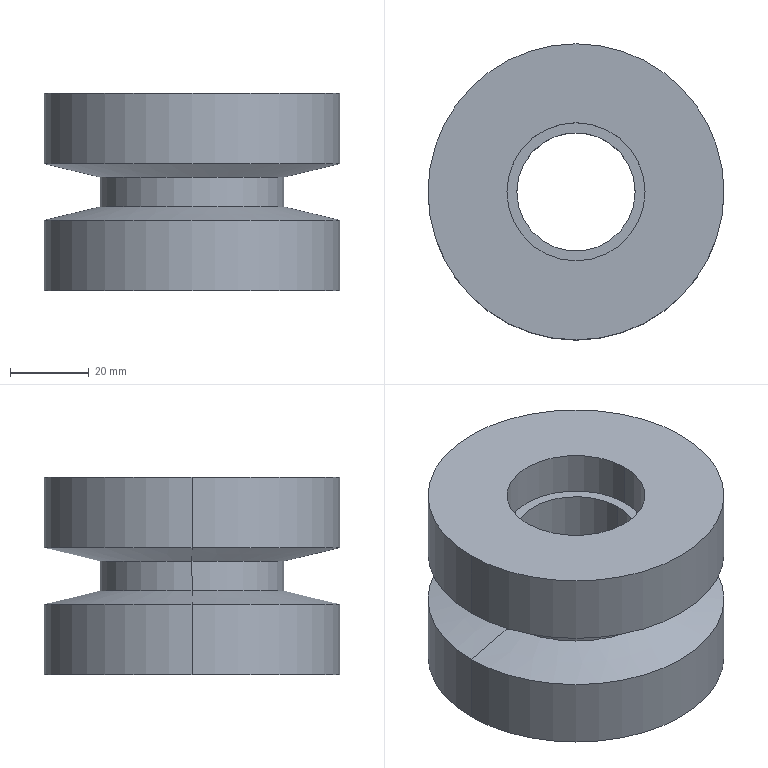Part | SolidWorks | features ICE 2, Extrusion 1, RevCut 1 | 1 solid | 20 faces | box 75 x 75 x 50 mm | volume 149506 mm3 | cylinder 12 | cone 4 | plane 4 | commonest cylinder face diameters 35 x4 75 x4 30 x2 46.5 x2
STEP:
#1=CARTESIAN_POINT('',(17.5,0.,11.));
#2=VERTEX_POINT('',#1);
#3=CARTESIAN_POINT('',(-17.5,0.,11.));
#4=VERTEX_POINT('',#3);
#5=CARTESIAN_POINT('',(0.,0.,11.));
#6=DIRECTION('',(0.,0.,-1.));
#7=DIRECTION('',(-1.,0.,0.));
#8=AXIS2_PLACEMENT_3D('',#5,#6,#7);
#9=CIRCLE('',#8,17.5);
#10=EDGE_CURVE('',#2,#4,#9,.T.);
#11=ORIENTED_EDGE('',*,*,#10,.F.);
#12=CARTESIAN_POINT('',(17.5,0.,0.));
#13=VERTEX_POINT('',#12);
#14=CARTESIAN_POINT('',(17.5,0.,11.));
#15=DIRECTION('',(0.,0.,-1.));
#16=VECTOR('',#15,1000.);
#17=LINE('',#14,#16);
#18=EDGE_CURVE('',#2,#13,#17,.T.);
#19=ORIENTED_EDGE('',*,*,#18,.T.);
#20=CARTESIAN_POINT('',(-17.5,0.,0.));
#21=VERTEX_POINT('',#20);
#22=CARTESIAN_POINT('',(0.,0.,0.));
#23=DIRECTION('',(0.,0.,-1.));
#24=DIRECTION('',(-1.,0.,0.));
#25=AXIS2_PLACEMENT_3D('',#22,#23,#24);
#26=CIRCLE('',#25,17.5);
#27=EDGE_CURVE('',#13,#21,#26,.T.);
#28=ORIENTED_EDGE('',*,*,#27,.T.);
#29=CARTESIAN_POINT('',(-17.5,0.,11.));
#30=DIRECTION('',(0.,0.,-1.));
#31=VECTOR('',#30,1000.);
#32=LINE('',#29,#31);
#33=EDGE_CURVE('',#4,#21,#32,.T.);
#34=ORIENTED_EDGE('',*,*,#33,.F.);
#35=EDGE_LOOP('',(#11,#19,#28,#34));
#36=FACE_OUTER_BOUND('',#35,.T.);
#37=CARTESIAN_POINT('',(0.,0.,11.));
#38=DIRECTION('',(0.,0.,-1.));
#39=DIRECTION('',(-1.,0.,0.));
#40=AXIS2_PLACEMENT_3D('',#37,#38,#39);
#41=CYLINDRICAL_SURFACE('',#40,17.5);
#42=ADVANCED_FACE('',(#36),#41,.F.);
#43=CARTESIAN_POINT('',(-17.5,0.,39.));
#44=VERTEX_POINT('',#43);
#45=CARTESIAN_POINT('',(17.5,0.,39.));
#46=VERTEX_POINT('',#45);
#47=CARTESIAN_POINT('',(0.,0.,39.));
#48=DIRECTION('',(0.,0.,1.));
#49=DIRECTION('',(1.,0.,0.));
#50=AXIS2_PLACEMENT_3D('',#47,#48,#49);
#51=CIRCLE('',#50,17.5);
#52=EDGE_CURVE('',#44,#46,#51,.T.);
#53=ORIENTED_EDGE('',*,*,#52,.F.);
#54=CARTESIAN_POINT('',(-17.5,0.,50.));
#55=VERTEX_POINT('',#54);
#56=CARTESIAN_POINT('',(-17.5,0.,39.));
#57=DIRECTION('',(0.,0.,1.));
#58=VECTOR('',#57,1000.);
#59=LINE('',#56,#58);
#60=EDGE_CURVE('',#44,#55,#59,.T.);
#61=ORIENTED_EDGE('',*,*,#60,.T.);
#62=CARTESIAN_POINT('',(17.5,0.,50.));
#63=VERTEX_POINT('',#62);
#64=CARTESIAN_POINT('',(0.,0.,50.));
#65=DIRECTION('',(0.,0.,1.));
#66=DIRECTION('',(1.,0.,0.));
#67=AXIS2_PLACEMENT_3D('',#64,#65,#66);
#68=CIRCLE('',#67,17.5);
#69=EDGE_CURVE('',#55,#63,#68,.T.);
#70=ORIENTED_EDGE('',*,*,#69,.T.);
#71=CARTESIAN_POINT('',(17.5,0.,39.));
#72=DIRECTION('',(0.,0.,1.));
#73=VECTOR('',#72,1000.);
#74=LINE('',#71,#73);
#75=EDGE_CURVE('',#46,#63,#74,.T.);
#76=ORIENTED_EDGE('',*,*,#75,.F.);
#77=EDGE_LOOP('',(#53,#61,#70,#76));
#78=FACE_OUTER_BOUND('',#77,.T.);
#79=CARTESIAN_POINT('',(0.,0.,39.));
#80=DIRECTION('',(0.,0.,1.));
#81=DIRECTION('',(1.,0.,0.));
#82=AXIS2_PLACEMENT_3D('',#79,#80,#81);
#83=CYLINDRICAL_SURFACE('',#82,17.5);
#84=ADVANCED_FACE('',(#78),#83,.F.);
#85=CARTESIAN_POINT('',(-23.25,0.,28.75));
#86=VERTEX_POINT('',#85);
#87=CARTESIAN_POINT('',(23.25,0.,28.75));
#88=VERTEX_POINT('',#87);
#89=CARTESIAN_POINT('',(0.,0.,28.75));
#90=DIRECTION('',(0.,0.,-1.));
#91=DIRECTION('',(-1.,0.,0.));
#92=AXIS2_PLACEMENT_3D('',#89,#90,#91);
#93=CIRCLE('',#92,23.25);
#94=EDGE_CURVE('',#86,#88,#93,.T.);
#95=ORIENTED_EDGE('',*,*,#94,.T.);
#96=CARTESIAN_POINT('',(23.25,0.,21.25));
#97=VERTEX_POINT('',#96);
#98=CARTESIAN_POINT('',(23.25,0.,0.));
#99=DIRECTION('',(0.,0.,-1.));
#100=VECTOR('',#99,1000.);
#101=LINE('',#98,#100);
#102=EDGE_CURVE('',#88,#97,#101,.T.);
#103=ORIENTED_EDGE('',*,*,#102,.T.);
#104=CARTESIAN_POINT('',(-23.25,0.,21.25));
#105=VERTEX_POINT('',#104);
#106=CARTESIAN_POINT('',(0.,0.,21.25));
#107=DIRECTION('',(0.,0.,-1.));
#108=DIRECTION('',(-1.,0.,0.));
#109=AXIS2_PLACEMENT_3D('',#106,#107,#108);
#110=CIRCLE('',#109,23.25);
#111=EDGE_CURVE('',#105,#97,#110,.T.);
#112=ORIENTED_EDGE('',*,*,#111,.F.);
#113=CARTESIAN_POINT('',(-23.25,0.,0.));
#114=DIRECTION('',(0.,0.,-1.));
#115=VECTOR('',#114,1000.);
#116=LINE('',#113,#115);
#117=EDGE_CURVE('',#86,#105,#116,.T.);
#118=ORIENTED_EDGE('',*,*,#117,.F.);
#119=EDGE_LOOP('',(#95,#103,#112,#118));
#120=FACE_OUTER_BOUND('',#119,.T.);
#121=CARTESIAN_POINT('',(0.,0.,0.));
#122=DIRECTION('',(0.,0.,-1.));
#123=DIRECTION('',(-1.,0.,0.));
#124=AXIS2_PLACEMENT_3D('',#121,#122,#123);
#125=CYLINDRICAL_SURFACE('',#124,23.25);
#126=ADVANCED_FACE('',(#120),#125,.T.);
#127=ORIENTED_EDGE('',*,*,#94,.F.);
#128=CARTESIAN_POINT('',(-37.5,0.,32.171));
#129=VERTEX_POINT('',#128);
#130=CARTESIAN_POINT('',(-38.25,0.,32.351));
#131=DIRECTION('',(-0.9724,0.,0.2334));
#132=VECTOR('',#131,1000.);
#133=LINE('',#130,#132);
#134=EDGE_CURVE('',#86,#129,#133,.T.);
#135=ORIENTED_EDGE('',*,*,#134,.T.);
#136=CARTESIAN_POINT('',(37.5,0.,32.171));
#137=VERTEX_POINT('',#136);
#138=CARTESIAN_POINT('',(0.,0.,32.171));
#139=DIRECTION('',(0.,0.,1.));
#140=DIRECTION('',(1.,0.,0.));
#141=AXIS2_PLACEMENT_3D('',#138,#139,#140);
#142=CIRCLE('',#141,37.5);
#143=EDGE_CURVE('',#137,#129,#142,.T.);
#144=ORIENTED_EDGE('',*,*,#143,.F.);
#145=CARTESIAN_POINT('',(38.25,0.,32.351));
#146=DIRECTION('',(0.9724,0.,0.2334));
#147=VECTOR('',#146,1000.);
#148=LINE('',#145,#147);
#149=EDGE_CURVE('',#88,#137,#148,.T.);
#150=ORIENTED_EDGE('',*,*,#149,.F.);
#151=EDGE_LOOP('',(#127,#135,#144,#150));
#152=FACE_OUTER_BOUND('',#151,.T.);
#153=CARTESIAN_POINT('',(0.,0.,32.351));
#154=DIRECTION('',(0.,0.,1.));
#155=DIRECTION('',(1.,0.,0.));
#156=AXIS2_PLACEMENT_3D('',#153,#154,#155);
#157=CONICAL_SURFACE('',#156,38.25,1.335);
#158=ADVANCED_FACE('',(#152),#157,.T.);
#159=ORIENTED_EDGE('',*,*,#111,.T.);
#160=CARTESIAN_POINT('',(37.5,0.,17.829));
#161=VERTEX_POINT('',#160);
#162=CARTESIAN_POINT('',(23.25,0.,21.25));
#163=DIRECTION('',(0.9724,0.,-0.2334));
#164=VECTOR('',#163,1000.);
#165=LINE('',#162,#164);
#166=EDGE_CURVE('',#97,#161,#165,.T.);
#167=ORIENTED_EDGE('',*,*,#166,.T.);
#168=CARTESIAN_POINT('',(-37.5,0.,17.829));
#169=VERTEX_POINT('',#168);
#170=CARTESIAN_POINT('',(0.,0.,17.829));
#171=DIRECTION('',(0.,0.,-1.));
#172=DIRECTION('',(-1.,0.,0.));
#173=AXIS2_PLACEMENT_3D('',#170,#171,#172);
#174=CIRCLE('',#173,37.5);
#175=EDGE_CURVE('',#169,#161,#174,.T.);
#176=ORIENTED_EDGE('',*,*,#175,.F.);
#177=CARTESIAN_POINT('',(-23.25,0.,21.25));
#178=DIRECTION('',(-0.9724,0.,-0.2334));
#179=VECTOR('',#178,1000.);
#180=LINE('',#177,#179);
#181=EDGE_CURVE('',#105,#169,#180,.T.);
#182=ORIENTED_EDGE('',*,*,#181,.F.);
#183=EDGE_LOOP('',(#159,#167,#176,#182));
#184=FACE_OUTER_BOUND('',#183,.T.);
#185=CARTESIAN_POINT('',(0.,0.,21.25));
#186=DIRECTION('',(0.,0.,-1.));
#187=DIRECTION('',(-1.,0.,0.));
#188=AXIS2_PLACEMENT_3D('',#185,#186,#187);
#189=CONICAL_SURFACE('',#188,23.25,1.335);
#190=ADVANCED_FACE('',(#184),#189,.T.);
#191=CARTESIAN_POINT('',(37.5,0.,50.));
#192=VERTEX_POINT('',#191);
#193=CARTESIAN_POINT('',(-37.5,0.,50.));
#194=VERTEX_POINT('',#193);
#195=CARTESIAN_POINT('',(0.,0.,50.));
#196=DIRECTION('',(0.,0.,1.));
#197=DIRECTION('',(1.,0.,0.));
#198=AXIS2_PLACEMENT_3D('',#195,#196,#197);
#199=CIRCLE('',#198,37.5);
#200=EDGE_CURVE('',#192,#194,#199,.T.);
#201=ORIENTED_EDGE('',*,*,#200,.F.);
#202=CARTESIAN_POINT('',(37.5,0.,50.));
#203=DIRECTION('',(0.,0.,-1.));
#204=VECTOR('',#203,1000.);
#205=LINE('',#202,#204);
#206=EDGE_CURVE('',#192,#137,#205,.T.);
#207=ORIENTED_EDGE('',*,*,#206,.T.);
#208=ORIENTED_EDGE('',*,*,#143,.T.);
#209=CARTESIAN_POINT('',(-37.5,0.,50.));
#210=DIRECTION('',(0.,0.,-1.));
#211=VECTOR('',#210,1000.);
#212=LINE('',#209,#211);
#213=EDGE_CURVE('',#194,#129,#212,.T.);
#214=ORIENTED_EDGE('',*,*,#213,.F.);
#215=EDGE_LOOP('',(#201,#207,#208,#214));
#216=FACE_OUTER_BOUND('',#215,.T.);
#217=CARTESIAN_POINT('',(0.,0.,50.));
#218=DIRECTION('',(0.,0.,-1.));
#219=DIRECTION('',(-1.,0.,0.));
#220=AXIS2_PLACEMENT_3D('',#217,#218,#219);
#221=CYLINDRICAL_SURFACE('',#220,37.5);
#222=ADVANCED_FACE('',(#216),#221,.T.);
#223=ORIENTED_EDGE('',*,*,#175,.T.);
#224=CARTESIAN_POINT('',(37.5,0.,0.));
#225=VERTEX_POINT('',#224);
#226=CARTESIAN_POINT('',(37.5,0.,50.));
#227=DIRECTION('',(0.,0.,-1.));
#228=VECTOR('',#227,1000.);
#229=LINE('',#226,#228);
#230=EDGE_CURVE('',#161,#225,#229,.T.);
#231=ORIENTED_EDGE('',*,*,#230,.T.);
#232=CARTESIAN_POINT('',(-37.5,0.,0.));
#233=VERTEX_POINT('',#232);
#234=CARTESIAN_POINT('',(0.,0.,0.));
#235=DIRECTION('',(0.,0.,1.));
#236=DIRECTION('',(1.,0.,0.));
#237=AXIS2_PLACEMENT_3D('',#234,#235,#236);
#238=CIRCLE('',#237,37.5);
#239=EDGE_CURVE('',#225,#233,#238,.T.);
#240=ORIENTED_EDGE('',*,*,#239,.T.);
#241=CARTESIAN_POINT('',(-37.5,0.,50.));
#242=DIRECTION('',(0.,0.,-1.));
#243=VECTOR('',#242,1000.);
#244=LINE('',#241,#243);
#245=EDGE_CURVE('',#169,#233,#244,.T.);
#246=ORIENTED_EDGE('',*,*,#245,.F.);
#247=EDGE_LOOP('',(#223,#231,#240,#246));
#248=FACE_OUTER_BOUND('',#247,.T.);
#249=CARTESIAN_POINT('',(0.,0.,50.));
#250=DIRECTION('',(0.,0.,-1.));
#251=DIRECTION('',(-1.,0.,0.));
#252=AXIS2_PLACEMENT_3D('',#249,#250,#251);
#253=CYLINDRICAL_SURFACE('',#252,37.5);
#254=ADVANCED_FACE('',(#248),#253,.T.);
#255=CARTESIAN_POINT('',(-15.,0.,39.));
#256=VERTEX_POINT('',#255);
#257=CARTESIAN_POINT('',(15.,0.,39.));
#258=VERTEX_POINT('',#257);
#259=CARTESIAN_POINT('',(0.,0.,39.));
#260=DIRECTION('',(0.,0.,1.));
#261=DIRECTION('',(1.,0.,0.));
#262=AXIS2_PLACEMENT_3D('',#259,#260,#261);
#263=CIRCLE('',#262,15.);
#264=EDGE_CURVE('',#256,#258,#263,.T.);
#265=ORIENTED_EDGE('',*,*,#264,.T.);
#266=CARTESIAN_POINT('',(15.,0.,11.));
#267=VERTEX_POINT('',#266);
#268=CARTESIAN_POINT('',(15.,0.,50.));
#269=DIRECTION('',(0.,0.,-1.));
#270=VECTOR('',#269,1000.);
#271=LINE('',#268,#270);
#272=EDGE_CURVE('',#258,#267,#271,.T.);
#273=ORIENTED_EDGE('',*,*,#272,.T.);
#274=CARTESIAN_POINT('',(-15.,0.,11.));
#275=VERTEX_POINT('',#274);
#276=CARTESIAN_POINT('',(0.,0.,11.));
#277=DIRECTION('',(0.,0.,-1.));
#278=DIRECTION('',(-1.,0.,0.));
#279=AXIS2_PLACEMENT_3D('',#276,#277,#278);
#280=CIRCLE('',#279,15.);
#281=EDGE_CURVE('',#267,#275,#280,.T.);
#282=ORIENTED_EDGE('',*,*,#281,.T.);
#283=CARTESIAN_POINT('',(-15.,0.,50.));
#284=DIRECTION('',(0.,0.,-1.));
#285=VECTOR('',#284,1000.);
#286=LINE('',#283,#285);
#287=EDGE_CURVE('',#256,#275,#286,.T.);
#288=ORIENTED_EDGE('',*,*,#287,.F.);
#289=EDGE_LOOP('',(#265,#273,#282,#288));
#290=FACE_OUTER_BOUND('',#289,.T.);
#291=CARTESIAN_POINT('',(0.,0.,50.));
#292=DIRECTION('',(0.,0.,-1.));
#293=DIRECTION('',(-1.,0.,0.));
#294=AXIS2_PLACEMENT_3D('',#291,#292,#293);
#295=CYLINDRICAL_SURFACE('',#294,15.);
#296=ADVANCED_FACE('',(#290),#295,.F.);
#297=ORIENTED_EDGE('',*,*,#272,.F.);
#298=CARTESIAN_POINT('',(0.,0.,39.));
#299=DIRECTION('',(0.,0.,1.));
#300=DIRECTION('',(1.,0.,0.));
#301=AXIS2_PLACEMENT_3D('',#298,#299,#300);
#302=CIRCLE('',#301,15.);
#303=EDGE_CURVE('',#258,#256,#302,.T.);
#304=ORIENTED_EDGE('',*,*,#303,.T.);
#305=ORIENTED_EDGE('',*,*,#287,.T.);
#306=CARTESIAN_POINT('',(0.,0.,11.));
#307=DIRECTION('',(0.,0.,-1.));
#308=DIRECTION('',(-1.,0.,0.));
#309=AXIS2_PLACEMENT_3D('',#306,#307,#308);
#310=CIRCLE('',#309,15.);
#311=EDGE_CURVE('',#275,#267,#310,.T.);
#312=ORIENTED_EDGE('',*,*,#311,.T.);
#313=EDGE_LOOP('',(#297,#304,#305,#312));
#314=FACE_OUTER_BOUND('',#313,.T.);
#315=CARTESIAN_POINT('',(0.,0.,50.));
#316=DIRECTION('',(0.,0.,-1.));
#317=DIRECTION('',(-1.,0.,0.));
#318=AXIS2_PLACEMENT_3D('',#315,#316,#317);
#319=CYLINDRICAL_SURFACE('',#318,15.);
#320=ADVANCED_FACE('',(#314),#319,.F.);
#321=ORIENTED_EDGE('',*,*,#230,.F.);
#322=CARTESIAN_POINT('',(0.,0.,17.829));
#323=DIRECTION('',(0.,0.,-1.));
#324=DIRECTION('',(-1.,0.,0.));
#325=AXIS2_PLACEMENT_3D('',#322,#323,#324);
#326=CIRCLE('',#325,37.5);
#327=EDGE_CURVE('',#161,#169,#326,.T.);
#328=ORIENTED_EDGE('',*,*,#327,.T.);
#329=ORIENTED_EDGE('',*,*,#245,.T.);
#330=CARTESIAN_POINT('',(0.,0.,0.));
#331=DIRECTION('',(0.,0.,1.));
#332=DIRECTION('',(1.,0.,0.));
#333=AXIS2_PLACEMENT_3D('',#330,#331,#332);
#334=CIRCLE('',#333,37.5);
#335=EDGE_CURVE('',#233,#225,#334,.T.);
#336=ORIENTED_EDGE('',*,*,#335,.T.);
#337=EDGE_LOOP('',(#321,#328,#329,#336));
#338=FACE_OUTER_BOUND('',#337,.T.);
#339=CARTESIAN_POINT('',(0.,0.,50.));
#340=DIRECTION('',(0.,0.,-1.));
#341=DIRECTION('',(-1.,0.,0.));
#342=AXIS2_PLACEMENT_3D('',#339,#340,#341);
#343=CYLINDRICAL_SURFACE('',#342,37.5);
#344=ADVANCED_FACE('',(#338),#343,.T.);
#345=CARTESIAN_POINT('',(0.,0.,50.));
#346=DIRECTION('',(0.,0.,1.));
#347=DIRECTION('',(1.,0.,0.));
#348=AXIS2_PLACEMENT_3D('',#345,#346,#347);
#349=CIRCLE('',#348,17.5);
#350=EDGE_CURVE('',#63,#55,#349,.T.);
#351=ORIENTED_EDGE('',*,*,#350,.F.);
#352=ORIENTED_EDGE('',*,*,#69,.F.);
#353=EDGE_LOOP('',(#351,#352));
#354=FACE_BOUND('',#353,.T.);
#355=CARTESIAN_POINT('',(0.,0.,50.));
#356=DIRECTION('',(0.,0.,1.));
#357=DIRECTION('',(1.,0.,0.));
#358=AXIS2_PLACEMENT_3D('',#355,#356,#357);
#359=CIRCLE('',#358,37.5);
#360=EDGE_CURVE('',#194,#192,#359,.T.);
#361=ORIENTED_EDGE('',*,*,#360,.T.);
#362=ORIENTED_EDGE('',*,*,#200,.T.);
#363=EDGE_LOOP('',(#361,#362));
#364=FACE_OUTER_BOUND('',#363,.T.);
#365=CARTESIAN_POINT('',(0.,0.,50.));
#366=DIRECTION('',(0.,0.,1.));
#367=DIRECTION('',(1.,0.,0.));
#368=AXIS2_PLACEMENT_3D('',#365,#366,#367);
#369=PLANE('',#368);
#370=ADVANCED_FACE('',(#354,#364),#369,.T.);
#371=CARTESIAN_POINT('',(0.,0.,0.));
#372=DIRECTION('',(0.,0.,-1.));
#373=DIRECTION('',(-1.,0.,0.));
#374=AXIS2_PLACEMENT_3D('',#371,#372,#373);
#375=CIRCLE('',#374,17.5);
#376=EDGE_CURVE('',#21,#13,#375,.T.);
#377=ORIENTED_EDGE('',*,*,#376,.F.);
#378=ORIENTED_EDGE('',*,*,#27,.F.);
#379=EDGE_LOOP('',(#377,#378));
#380=FACE_BOUND('',#379,.T.);
#381=ORIENTED_EDGE('',*,*,#335,.F.);
#382=ORIENTED_EDGE('',*,*,#239,.F.);
#383=EDGE_LOOP('',(#381,#382));
#384=FACE_OUTER_BOUND('',#383,.T.);
#385=CARTESIAN_POINT('',(0.,0.,0.));
#386=DIRECTION('',(0.,0.,1.));
#387=DIRECTION('',(1.,0.,0.));
#388=AXIS2_PLACEMENT_3D('',#385,#386,#387);
#389=PLANE('',#388);
#390=ADVANCED_FACE('',(#380,#384),#389,.F.);
#391=ORIENTED_EDGE('',*,*,#206,.F.);
#392=ORIENTED_EDGE('',*,*,#360,.F.);
#393=ORIENTED_EDGE('',*,*,#213,.T.);
#394=CARTESIAN_POINT('',(0.,0.,32.171));
#395=DIRECTION('',(0.,0.,1.));
#396=DIRECTION('',(1.,0.,0.));
#397=AXIS2_PLACEMENT_3D('',#394,#395,#396);
#398=CIRCLE('',#397,37.5);
#399=EDGE_CURVE('',#129,#137,#398,.T.);
#400=ORIENTED_EDGE('',*,*,#399,.T.);
#401=EDGE_LOOP('',(#391,#392,#393,#400));
#402=FACE_OUTER_BOUND('',#401,.T.);
#403=CARTESIAN_POINT('',(0.,0.,50.));
#404=DIRECTION('',(0.,0.,-1.));
#405=DIRECTION('',(-1.,0.,0.));
#406=AXIS2_PLACEMENT_3D('',#403,#404,#405);
#407=CYLINDRICAL_SURFACE('',#406,37.5);
#408=ADVANCED_FACE('',(#402),#407,.T.);
#409=ORIENTED_EDGE('',*,*,#166,.F.);
#410=CARTESIAN_POINT('',(0.,0.,21.25));
#411=DIRECTION('',(0.,0.,-1.));
#412=DIRECTION('',(-1.,0.,0.));
#413=AXIS2_PLACEMENT_3D('',#410,#411,#412);
#414=CIRCLE('',#413,23.25);
#415=EDGE_CURVE('',#97,#105,#414,.T.);
#416=ORIENTED_EDGE('',*,*,#415,.T.);
#417=ORIENTED_EDGE('',*,*,#181,.T.);
#418=ORIENTED_EDGE('',*,*,#327,.F.);
#419=EDGE_LOOP('',(#409,#416,#417,#418));
#420=FACE_OUTER_BOUND('',#419,.T.);
#421=CARTESIAN_POINT('',(0.,0.,21.25));
#422=DIRECTION('',(0.,0.,-1.));
#423=DIRECTION('',(-1.,0.,0.));
#424=AXIS2_PLACEMENT_3D('',#421,#422,#423);
#425=CONICAL_SURFACE('',#424,23.25,1.335);
#426=ADVANCED_FACE('',(#420),#425,.T.);
#427=ORIENTED_EDGE('',*,*,#134,.F.);
#428=CARTESIAN_POINT('',(0.,0.,28.75));
#429=DIRECTION('',(0.,0.,-1.));
#430=DIRECTION('',(-1.,0.,0.));
#431=AXIS2_PLACEMENT_3D('',#428,#429,#430);
#432=CIRCLE('',#431,23.25);
#433=EDGE_CURVE('',#88,#86,#432,.T.);
#434=ORIENTED_EDGE('',*,*,#433,.F.);
#435=ORIENTED_EDGE('',*,*,#149,.T.);
#436=ORIENTED_EDGE('',*,*,#399,.F.);
#437=EDGE_LOOP('',(#427,#434,#435,#436));
#438=FACE_OUTER_BOUND('',#437,.T.);
#439=CARTESIAN_POINT('',(0.,0.,32.351));
#440=DIRECTION('',(0.,0.,1.));
#441=DIRECTION('',(1.,0.,0.));
#442=AXIS2_PLACEMENT_3D('',#439,#440,#441);
#443=CONICAL_SURFACE('',#442,38.25,1.335);
#444=ADVANCED_FACE('',(#438),#443,.T.);
#445=ORIENTED_EDGE('',*,*,#102,.F.);
#446=ORIENTED_EDGE('',*,*,#433,.T.);
#447=ORIENTED_EDGE('',*,*,#117,.T.);
#448=ORIENTED_EDGE('',*,*,#415,.F.);
#449=EDGE_LOOP('',(#445,#446,#447,#448));
#450=FACE_OUTER_BOUND('',#449,.T.);
#451=CARTESIAN_POINT('',(0.,0.,0.));
#452=DIRECTION('',(0.,0.,-1.));
#453=DIRECTION('',(-1.,0.,0.));
#454=AXIS2_PLACEMENT_3D('',#451,#452,#453);
#455=CYLINDRICAL_SURFACE('',#454,23.25);
#456=ADVANCED_FACE('',(#450),#455,.T.);
#457=ORIENTED_EDGE('',*,*,#60,.F.);
#458=CARTESIAN_POINT('',(0.,0.,39.));
#459=DIRECTION('',(0.,0.,1.));
#460=DIRECTION('',(1.,0.,0.));
#461=AXIS2_PLACEMENT_3D('',#458,#459,#460);
#462=CIRCLE('',#461,17.5);
#463=EDGE_CURVE('',#46,#44,#462,.T.);
#464=ORIENTED_EDGE('',*,*,#463,.F.);
#465=ORIENTED_EDGE('',*,*,#75,.T.);
#466=ORIENTED_EDGE('',*,*,#350,.T.);
#467=EDGE_LOOP('',(#457,#464,#465,#466));
#468=FACE_OUTER_BOUND('',#467,.T.);
#469=CARTESIAN_POINT('',(0.,0.,39.));
#470=DIRECTION('',(0.,0.,1.));
#471=DIRECTION('',(1.,0.,0.));
#472=AXIS2_PLACEMENT_3D('',#469,#470,#471);
#473=CYLINDRICAL_SURFACE('',#472,17.5);
#474=ADVANCED_FACE('',(#468),#473,.F.);
#475=ORIENTED_EDGE('',*,*,#264,.F.);
#476=ORIENTED_EDGE('',*,*,#303,.F.);
#477=EDGE_LOOP('',(#475,#476));
#478=FACE_BOUND('',#477,.T.);
#479=ORIENTED_EDGE('',*,*,#463,.T.);
#480=ORIENTED_EDGE('',*,*,#52,.T.);
#481=EDGE_LOOP('',(#479,#480));
#482=FACE_OUTER_BOUND('',#481,.T.);
#483=CARTESIAN_POINT('',(0.,0.,39.));
#484=DIRECTION('',(0.,0.,1.));
#485=DIRECTION('',(1.,0.,0.));
#486=AXIS2_PLACEMENT_3D('',#483,#484,#485);
#487=PLANE('',#486);
#488=ADVANCED_FACE('',(#478,#482),#487,.T.);
#489=ORIENTED_EDGE('',*,*,#18,.F.);
#490=CARTESIAN_POINT('',(0.,0.,11.));
#491=DIRECTION('',(0.,0.,-1.));
#492=DIRECTION('',(-1.,0.,0.));
#493=AXIS2_PLACEMENT_3D('',#490,#491,#492);
#494=CIRCLE('',#493,17.5);
#495=EDGE_CURVE('',#4,#2,#494,.T.);
#496=ORIENTED_EDGE('',*,*,#495,.F.);
#497=ORIENTED_EDGE('',*,*,#33,.T.);
#498=ORIENTED_EDGE('',*,*,#376,.T.);
#499=EDGE_LOOP('',(#489,#496,#497,#498));
#500=FACE_OUTER_BOUND('',#499,.T.);
#501=CARTESIAN_POINT('',(0.,0.,11.));
#502=DIRECTION('',(0.,0.,-1.));
#503=DIRECTION('',(-1.,0.,0.));
#504=AXIS2_PLACEMENT_3D('',#501,#502,#503);
#505=CYLINDRICAL_SURFACE('',#504,17.5);
#506=ADVANCED_FACE('',(#500),#505,.F.);
#507=ORIENTED_EDGE('',*,*,#311,.F.);
#508=ORIENTED_EDGE('',*,*,#281,.F.);
#509=EDGE_LOOP('',(#507,#508));
#510=FACE_BOUND('',#509,.T.);
#511=ORIENTED_EDGE('',*,*,#495,.T.);
#512=ORIENTED_EDGE('',*,*,#10,.T.);
#513=EDGE_LOOP('',(#511,#512));
#514=FACE_OUTER_BOUND('',#513,.T.);
#515=CARTESIAN_POINT('',(0.,0.,11.));
#516=DIRECTION('',(0.,0.,-1.));
#517=DIRECTION('',(-1.,0.,0.));
#518=AXIS2_PLACEMENT_3D('',#515,#516,#517);
#519=PLANE('',#518);
#520=ADVANCED_FACE('',(#510,#514),#519,.T.);
#521=CLOSED_SHELL('',(#42,#84,#126,#158,#190,#222,#254,#296,#320,#344,#370,#390,#408,#426,#444,#456,#474,#488,#506,#520));
#522=MANIFOLD_SOLID_BREP('',#521);
#523=CARTESIAN_POINT('',(0.,0.,0.));
#524=DIRECTION('',(0.,0.,1.));
#525=DIRECTION('',(1.,0.,0.));
#526=AXIS2_PLACEMENT_3D('',#523,#524,#525);
#527=(LENGTH_UNIT()NAMED_UNIT(*)SI_UNIT(.MILLI.,.METRE.));
#528=UNCERTAINTY_MEASURE_WITH_UNIT(LENGTH_MEASURE(0.00001),#527,'','');
#529=(NAMED_UNIT(*)PLANE_ANGLE_UNIT()SI_UNIT($,.RADIAN.));
#530=(NAMED_UNIT(*)SI_UNIT($,.STERADIAN.)SOLID_ANGLE_UNIT());
#531=(GEOMETRIC_REPRESENTATION_CONTEXT(3)GLOBAL_UNCERTAINTY_ASSIGNED_CONTEXT((#528))GLOBAL_UNIT_ASSIGNED_CONTEXT((#527,#529,#530))REPRESENTATION_CONTEXT('',''));
#532=ADVANCED_BREP_SHAPE_REPRESENTATION('',(#522,#526),#531);